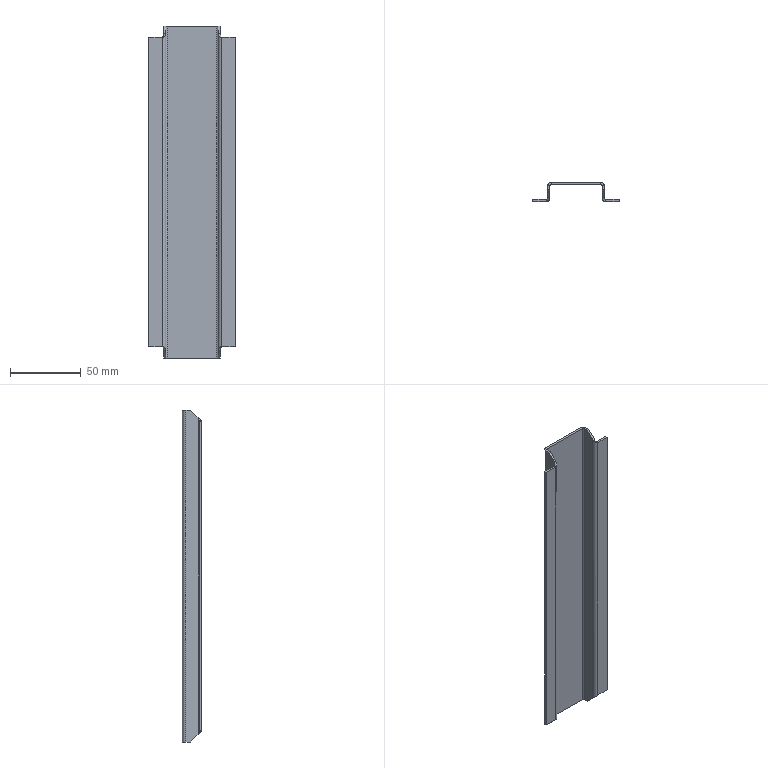Part | SolidWorks | features FlatPattern 1, ICE 1, SMBaseFlange 1, SheetMetal 1 | 1 solid | 42 faces | box 61 x 13.5 x 234.5 mm | volume 28178 mm3 | plane 30 | cylinder 8 | spline 4 | commonest cylinder face diameters 2 x4 5 x4
STEP:
#1=CARTESIAN_POINT('',(22.477,31.708,8.));
#2=VERTEX_POINT('',#1);
#3=CARTESIAN_POINT('',(12.977,31.708,8.));
#4=VERTEX_POINT('',#3);
#5=CARTESIAN_POINT('',(168.477,31.708,8.));
#6=DIRECTION('',(-1.,0.,0.));
#7=VECTOR('',#6,1000.);
#8=LINE('',#5,#7);
#9=EDGE_CURVE('',#2,#4,#8,.T.);
#10=ORIENTED_EDGE('',*,*,#9,.F.);
#11=CARTESIAN_POINT('',(22.477,31.708,226.5));
#12=VERTEX_POINT('',#11);
#13=CARTESIAN_POINT('',(22.477,31.708,234.5));
#14=DIRECTION('',(0.,0.,-1.));
#15=VECTOR('',#14,1000.);
#16=LINE('',#13,#15);
#17=EDGE_CURVE('',#12,#2,#16,.T.);
#18=ORIENTED_EDGE('',*,*,#17,.F.);
#19=CARTESIAN_POINT('',(12.977,31.708,226.5));
#20=VERTEX_POINT('',#19);
#21=CARTESIAN_POINT('',(168.477,31.708,226.5));
#22=DIRECTION('',(-1.,0.,0.));
#23=VECTOR('',#22,1000.);
#24=LINE('',#21,#23);
#25=EDGE_CURVE('',#12,#20,#24,.T.);
#26=ORIENTED_EDGE('',*,*,#25,.T.);
#27=CARTESIAN_POINT('',(12.977,31.708,234.5));
#28=DIRECTION('',(0.,0.,-1.));
#29=VECTOR('',#28,1000.);
#30=LINE('',#27,#29);
#31=EDGE_CURVE('',#20,#4,#30,.T.);
#32=ORIENTED_EDGE('',*,*,#31,.T.);
#33=EDGE_LOOP('',(#10,#18,#26,#32));
#34=FACE_OUTER_BOUND('',#33,.T.);
#35=CARTESIAN_POINT('',(11.977,31.708,234.5));
#36=DIRECTION('',(0.,1.,0.));
#37=DIRECTION('',(0.,0.,1.));
#38=AXIS2_PLACEMENT_3D('',#35,#36,#37);
#39=PLANE('',#38);
#40=ADVANCED_FACE('',(#34),#39,.F.);
#41=ORIENTED_EDGE('',*,*,#17,.T.);
#42=CARTESIAN_POINT('',(22.477,33.208,8.));
#43=VERTEX_POINT('',#42);
#44=CARTESIAN_POINT('',(22.477,31.708,8.));
#45=DIRECTION('',(0.,1.,0.));
#46=VECTOR('',#45,1000.);
#47=LINE('',#44,#46);
#48=EDGE_CURVE('',#2,#43,#47,.T.);
#49=ORIENTED_EDGE('',*,*,#48,.T.);
#50=CARTESIAN_POINT('',(22.477,33.208,226.5));
#51=VERTEX_POINT('',#50);
#52=CARTESIAN_POINT('',(22.477,33.208,234.5));
#53=DIRECTION('',(0.,0.,-1.));
#54=VECTOR('',#53,1000.);
#55=LINE('',#52,#54);
#56=EDGE_CURVE('',#51,#43,#55,.T.);
#57=ORIENTED_EDGE('',*,*,#56,.F.);
#58=CARTESIAN_POINT('',(22.477,31.708,226.5));
#59=DIRECTION('',(0.,1.,0.));
#60=VECTOR('',#59,1000.);
#61=LINE('',#58,#60);
#62=EDGE_CURVE('',#12,#51,#61,.T.);
#63=ORIENTED_EDGE('',*,*,#62,.F.);
#64=EDGE_LOOP('',(#41,#49,#57,#63));
#65=FACE_OUTER_BOUND('',#64,.T.);
#66=CARTESIAN_POINT('',(22.477,33.208,234.5));
#67=DIRECTION('',(1.,0.,0.));
#68=DIRECTION('',(0.,0.,-1.));
#69=AXIS2_PLACEMENT_3D('',#66,#67,#68);
#70=PLANE('',#69);
#71=ADVANCED_FACE('',(#65),#70,.T.);
#72=ORIENTED_EDGE('',*,*,#56,.T.);
#73=CARTESIAN_POINT('',(12.977,33.208,8.));
#74=VERTEX_POINT('',#73);
#75=CARTESIAN_POINT('',(11.977,33.208,8.));
#76=DIRECTION('',(-1.,0.,0.));
#77=VECTOR('',#76,1000.);
#78=LINE('',#75,#77);
#79=EDGE_CURVE('',#43,#74,#78,.T.);
#80=ORIENTED_EDGE('',*,*,#79,.T.);
#81=CARTESIAN_POINT('',(12.977,33.208,226.5));
#82=VERTEX_POINT('',#81);
#83=CARTESIAN_POINT('',(12.977,33.208,234.5));
#84=DIRECTION('',(0.,0.,-1.));
#85=VECTOR('',#84,1000.);
#86=LINE('',#83,#85);
#87=EDGE_CURVE('',#82,#74,#86,.T.);
#88=ORIENTED_EDGE('',*,*,#87,.F.);
#89=CARTESIAN_POINT('',(11.977,33.208,226.5));
#90=DIRECTION('',(-1.,0.,0.));
#91=VECTOR('',#90,1000.);
#92=LINE('',#89,#91);
#93=EDGE_CURVE('',#51,#82,#92,.T.);
#94=ORIENTED_EDGE('',*,*,#93,.F.);
#95=EDGE_LOOP('',(#72,#80,#88,#94));
#96=FACE_OUTER_BOUND('',#95,.T.);
#97=CARTESIAN_POINT('',(11.977,33.208,234.5));
#98=DIRECTION('',(0.,1.,0.));
#99=DIRECTION('',(0.,0.,1.));
#100=AXIS2_PLACEMENT_3D('',#97,#98,#99);
#101=PLANE('',#100);
#102=ADVANCED_FACE('',(#96),#101,.T.);
#103=ORIENTED_EDGE('',*,*,#87,.T.);
#104=CARTESIAN_POINT('',(11.977,34.208,5.5));
#105=VERTEX_POINT('',#104);
#106=CARTESIAN_POINT('',(11.977,34.208,5.5));
#107=CARTESIAN_POINT('',(11.977,33.623,6.964));
#108=CARTESIAN_POINT('',(12.391,33.208,8.));
#109=CARTESIAN_POINT('',(12.977,33.208,8.));
#110=(BOUNDED_CURVE()B_SPLINE_CURVE(3,(#106,#107,#108,#109),.UNSPECIFIED.,.F.,.F.)B_SPLINE_CURVE_WITH_KNOTS((4,4),(1.571,3.142),.UNSPECIFIED.)CURVE()GEOMETRIC_REPRESENTATION_ITEM()RATIONAL_B_SPLINE_CURVE((1.,0.8047,0.8047,1.))REPRESENTATION_ITEM(''));
#111=EDGE_CURVE('',#105,#74,#110,.T.);
#112=ORIENTED_EDGE('',*,*,#111,.F.);
#113=CARTESIAN_POINT('',(11.977,34.208,229.));
#114=VERTEX_POINT('',#113);
#115=CARTESIAN_POINT('',(11.977,34.208,234.5));
#116=DIRECTION('',(0.,0.,-1.));
#117=VECTOR('',#116,1000.);
#118=LINE('',#115,#117);
#119=EDGE_CURVE('',#114,#105,#118,.T.);
#120=ORIENTED_EDGE('',*,*,#119,.F.);
#121=CARTESIAN_POINT('',(12.977,33.208,226.5));
#122=CARTESIAN_POINT('',(12.391,33.208,226.5));
#123=CARTESIAN_POINT('',(11.977,33.623,227.536));
#124=CARTESIAN_POINT('',(11.977,34.208,229.));
#125=(BOUNDED_CURVE()B_SPLINE_CURVE(3,(#121,#122,#123,#124),.UNSPECIFIED.,.F.,.T.)B_SPLINE_CURVE_WITH_KNOTS((4,4),(0.,1.571),.UNSPECIFIED.)CURVE()GEOMETRIC_REPRESENTATION_ITEM()RATIONAL_B_SPLINE_CURVE((1.,0.8047,0.8047,1.))REPRESENTATION_ITEM(''));
#126=EDGE_CURVE('',#82,#114,#125,.T.);
#127=ORIENTED_EDGE('',*,*,#126,.F.);
#128=EDGE_LOOP('',(#103,#112,#120,#127));
#129=FACE_OUTER_BOUND('',#128,.T.);
#130=CARTESIAN_POINT('',(12.977,34.208,234.5));
#131=DIRECTION('',(0.,0.,-1.));
#132=DIRECTION('',(-1.,0.,0.));
#133=AXIS2_PLACEMENT_3D('',#130,#131,#132);
#134=CYLINDRICAL_SURFACE('',#133,1.);
#135=ADVANCED_FACE('',(#129),#134,.F.);
#136=ORIENTED_EDGE('',*,*,#119,.T.);
#137=CARTESIAN_POINT('',(11.977,39.708,0.));
#138=VERTEX_POINT('',#137);
#139=CARTESIAN_POINT('',(11.977,-74.792,114.5));
#140=DIRECTION('',(0.,-0.7071,0.7071));
#141=VECTOR('',#140,1000.);
#142=LINE('',#139,#141);
#143=EDGE_CURVE('',#138,#105,#142,.T.);
#144=ORIENTED_EDGE('',*,*,#143,.F.);
#145=CARTESIAN_POINT('',(11.977,42.708,0.));
#146=VERTEX_POINT('',#145);
#147=CARTESIAN_POINT('',(11.977,45.208,0.));
#148=DIRECTION('',(0.,-1.,0.));
#149=VECTOR('',#148,1000.);
#150=LINE('',#147,#149);
#151=EDGE_CURVE('',#146,#138,#150,.T.);
#152=ORIENTED_EDGE('',*,*,#151,.F.);
#153=CARTESIAN_POINT('',(11.977,42.708,234.5));
#154=VERTEX_POINT('',#153);
#155=CARTESIAN_POINT('',(11.977,42.708,234.5));
#156=DIRECTION('',(0.,0.,-1.));
#157=VECTOR('',#156,1000.);
#158=LINE('',#155,#157);
#159=EDGE_CURVE('',#154,#146,#158,.T.);
#160=ORIENTED_EDGE('',*,*,#159,.F.);
#161=CARTESIAN_POINT('',(11.977,39.708,234.5));
#162=VERTEX_POINT('',#161);
#163=CARTESIAN_POINT('',(11.977,45.208,234.5));
#164=DIRECTION('',(0.,-1.,0.));
#165=VECTOR('',#164,1000.);
#166=LINE('',#163,#165);
#167=EDGE_CURVE('',#154,#162,#166,.T.);
#168=ORIENTED_EDGE('',*,*,#167,.T.);
#169=CARTESIAN_POINT('',(11.977,42.458,237.25));
#170=DIRECTION('',(0.,0.7071,0.7071));
#171=VECTOR('',#170,1000.);
#172=LINE('',#169,#171);
#173=EDGE_CURVE('',#114,#162,#172,.T.);
#174=ORIENTED_EDGE('',*,*,#173,.F.);
#175=EDGE_LOOP('',(#136,#144,#152,#160,#168,#174));
#176=FACE_OUTER_BOUND('',#175,.T.);
#177=CARTESIAN_POINT('',(11.977,45.208,234.5));
#178=DIRECTION('',(1.,0.,0.));
#179=DIRECTION('',(0.,1.,0.));
#180=AXIS2_PLACEMENT_3D('',#177,#178,#179);
#181=PLANE('',#180);
#182=ADVANCED_FACE('',(#176),#181,.T.);
#183=CARTESIAN_POINT('',(10.477,39.708,0.));
#184=VERTEX_POINT('',#183);
#185=CARTESIAN_POINT('',(10.477,34.208,5.5));
#186=VERTEX_POINT('',#185);
#187=CARTESIAN_POINT('',(10.477,-74.792,114.5));
#188=DIRECTION('',(0.,-0.7071,0.7071));
#189=VECTOR('',#188,1000.);
#190=LINE('',#187,#189);
#191=EDGE_CURVE('',#184,#186,#190,.T.);
#192=ORIENTED_EDGE('',*,*,#191,.T.);
#193=CARTESIAN_POINT('',(10.477,34.208,229.));
#194=VERTEX_POINT('',#193);
#195=CARTESIAN_POINT('',(10.477,34.208,234.5));
#196=DIRECTION('',(0.,0.,-1.));
#197=VECTOR('',#196,1000.);
#198=LINE('',#195,#197);
#199=EDGE_CURVE('',#194,#186,#198,.T.);
#200=ORIENTED_EDGE('',*,*,#199,.F.);
#201=CARTESIAN_POINT('',(10.477,39.708,234.5));
#202=VERTEX_POINT('',#201);
#203=CARTESIAN_POINT('',(10.477,42.458,237.25));
#204=DIRECTION('',(0.,0.7071,0.7071));
#205=VECTOR('',#204,1000.);
#206=LINE('',#203,#205);
#207=EDGE_CURVE('',#194,#202,#206,.T.);
#208=ORIENTED_EDGE('',*,*,#207,.T.);
#209=CARTESIAN_POINT('',(10.477,42.708,234.5));
#210=VERTEX_POINT('',#209);
#211=CARTESIAN_POINT('',(10.477,45.208,234.5));
#212=DIRECTION('',(0.,-1.,0.));
#213=VECTOR('',#212,1000.);
#214=LINE('',#211,#213);
#215=EDGE_CURVE('',#210,#202,#214,.T.);
#216=ORIENTED_EDGE('',*,*,#215,.F.);
#217=CARTESIAN_POINT('',(10.477,42.708,0.));
#218=VERTEX_POINT('',#217);
#219=CARTESIAN_POINT('',(10.477,42.708,234.5));
#220=DIRECTION('',(0.,0.,-1.));
#221=VECTOR('',#220,1000.);
#222=LINE('',#219,#221);
#223=EDGE_CURVE('',#210,#218,#222,.T.);
#224=ORIENTED_EDGE('',*,*,#223,.T.);
#225=CARTESIAN_POINT('',(10.477,45.208,0.));
#226=DIRECTION('',(0.,-1.,0.));
#227=VECTOR('',#226,1000.);
#228=LINE('',#225,#227);
#229=EDGE_CURVE('',#218,#184,#228,.T.);
#230=ORIENTED_EDGE('',*,*,#229,.T.);
#231=EDGE_LOOP('',(#192,#200,#208,#216,#224,#230));
#232=FACE_OUTER_BOUND('',#231,.T.);
#233=CARTESIAN_POINT('',(10.477,45.208,234.5));
#234=DIRECTION('',(1.,0.,0.));
#235=DIRECTION('',(0.,1.,0.));
#236=AXIS2_PLACEMENT_3D('',#233,#234,#235);
#237=PLANE('',#236);
#238=ADVANCED_FACE('',(#232),#237,.F.);
#239=CARTESIAN_POINT('',(10.477,34.208,5.5));
#240=CARTESIAN_POINT('',(10.477,32.744,6.964));
#241=CARTESIAN_POINT('',(11.512,31.708,8.));
#242=CARTESIAN_POINT('',(12.977,31.708,8.));
#243=(BOUNDED_CURVE()B_SPLINE_CURVE(3,(#239,#240,#241,#242),.UNSPECIFIED.,.F.,.F.)B_SPLINE_CURVE_WITH_KNOTS((4,4),(1.571,3.142),.UNSPECIFIED.)CURVE()GEOMETRIC_REPRESENTATION_ITEM()RATIONAL_B_SPLINE_CURVE((1.,0.8047,0.8047,1.))REPRESENTATION_ITEM(''));
#244=EDGE_CURVE('',#186,#4,#243,.T.);
#245=ORIENTED_EDGE('',*,*,#244,.T.);
#246=ORIENTED_EDGE('',*,*,#31,.F.);
#247=CARTESIAN_POINT('',(12.977,31.708,226.5));
#248=CARTESIAN_POINT('',(11.512,31.708,226.5));
#249=CARTESIAN_POINT('',(10.477,32.744,227.536));
#250=CARTESIAN_POINT('',(10.477,34.208,229.));
#251=(BOUNDED_CURVE()B_SPLINE_CURVE(3,(#247,#248,#249,#250),.UNSPECIFIED.,.F.,.F.)B_SPLINE_CURVE_WITH_KNOTS((4,4),(0.,1.571),.UNSPECIFIED.)CURVE()GEOMETRIC_REPRESENTATION_ITEM()RATIONAL_B_SPLINE_CURVE((1.,0.8047,0.8047,1.))REPRESENTATION_ITEM(''));
#252=EDGE_CURVE('',#20,#194,#251,.T.);
#253=ORIENTED_EDGE('',*,*,#252,.T.);
#254=ORIENTED_EDGE('',*,*,#199,.T.);
#255=EDGE_LOOP('',(#245,#246,#253,#254));
#256=FACE_OUTER_BOUND('',#255,.T.);
#257=CARTESIAN_POINT('',(12.977,34.208,234.5));
#258=DIRECTION('',(0.,0.,-1.));
#259=DIRECTION('',(-1.,0.,0.));
#260=AXIS2_PLACEMENT_3D('',#257,#258,#259);
#261=CYLINDRICAL_SURFACE('',#260,2.5);
#262=ADVANCED_FACE('',(#256),#261,.T.);
#263=CARTESIAN_POINT('',(-28.023,39.708,0.));
#264=VERTEX_POINT('',#263);
#265=CARTESIAN_POINT('',(-28.023,42.708,0.));
#266=VERTEX_POINT('',#265);
#267=CARTESIAN_POINT('',(-28.023,33.208,0.));
#268=DIRECTION('',(0.,1.,0.));
#269=VECTOR('',#268,1000.);
#270=LINE('',#267,#269);
#271=EDGE_CURVE('',#264,#266,#270,.T.);
#272=ORIENTED_EDGE('',*,*,#271,.F.);
#273=CARTESIAN_POINT('',(-28.023,34.208,5.5));
#274=VERTEX_POINT('',#273);
#275=CARTESIAN_POINT('',(-28.023,-80.792,120.5));
#276=DIRECTION('',(0.,0.7071,-0.7071));
#277=VECTOR('',#276,1000.);
#278=LINE('',#275,#277);
#279=EDGE_CURVE('',#274,#264,#278,.T.);
#280=ORIENTED_EDGE('',*,*,#279,.F.);
#281=CARTESIAN_POINT('',(-28.023,34.208,229.));
#282=VERTEX_POINT('',#281);
#283=CARTESIAN_POINT('',(-28.023,34.208,234.5));
#284=DIRECTION('',(0.,0.,-1.));
#285=VECTOR('',#284,1000.);
#286=LINE('',#283,#285);
#287=EDGE_CURVE('',#282,#274,#286,.T.);
#288=ORIENTED_EDGE('',*,*,#287,.F.);
#289=CARTESIAN_POINT('',(-28.023,39.708,234.5));
#290=VERTEX_POINT('',#289);
#291=CARTESIAN_POINT('',(-28.023,36.458,231.25));
#292=DIRECTION('',(0.,-0.7071,-0.7071));
#293=VECTOR('',#292,1000.);
#294=LINE('',#291,#293);
#295=EDGE_CURVE('',#290,#282,#294,.T.);
#296=ORIENTED_EDGE('',*,*,#295,.F.);
#297=CARTESIAN_POINT('',(-28.023,42.708,234.5));
#298=VERTEX_POINT('',#297);
#299=CARTESIAN_POINT('',(-28.023,33.208,234.5));
#300=DIRECTION('',(0.,1.,0.));
#301=VECTOR('',#300,1000.);
#302=LINE('',#299,#301);
#303=EDGE_CURVE('',#290,#298,#302,.T.);
#304=ORIENTED_EDGE('',*,*,#303,.T.);
#305=CARTESIAN_POINT('',(-28.023,42.708,234.5));
#306=DIRECTION('',(0.,0.,-1.));
#307=VECTOR('',#306,1000.);
#308=LINE('',#305,#307);
#309=EDGE_CURVE('',#298,#266,#308,.T.);
#310=ORIENTED_EDGE('',*,*,#309,.T.);
#311=EDGE_LOOP('',(#272,#280,#288,#296,#304,#310));
#312=FACE_OUTER_BOUND('',#311,.T.);
#313=CARTESIAN_POINT('',(-28.023,33.208,234.5));
#314=DIRECTION('',(-1.,0.,0.));
#315=DIRECTION('',(0.,0.,1.));
#316=AXIS2_PLACEMENT_3D('',#313,#314,#315);
#317=PLANE('',#316);
#318=ADVANCED_FACE('',(#312),#317,.T.);
#319=ORIENTED_EDGE('',*,*,#287,.T.);
#320=CARTESIAN_POINT('',(-29.023,33.208,8.));
#321=VERTEX_POINT('',#320);
#322=CARTESIAN_POINT('',(-29.023,33.208,8.));
#323=CARTESIAN_POINT('',(-28.437,33.208,8.));
#324=CARTESIAN_POINT('',(-28.023,33.623,6.964));
#325=CARTESIAN_POINT('',(-28.023,34.208,5.5));
#326=(BOUNDED_CURVE()B_SPLINE_CURVE(3,(#322,#323,#324,#325),.UNSPECIFIED.,.F.,.F.)B_SPLINE_CURVE_WITH_KNOTS((4,4),(3.142,4.712),.UNSPECIFIED.)CURVE()GEOMETRIC_REPRESENTATION_ITEM()RATIONAL_B_SPLINE_CURVE((1.,0.8047,0.8047,1.))REPRESENTATION_ITEM(''));
#327=EDGE_CURVE('',#321,#274,#326,.T.);
#328=ORIENTED_EDGE('',*,*,#327,.F.);
#329=CARTESIAN_POINT('',(-29.023,33.208,226.5));
#330=VERTEX_POINT('',#329);
#331=CARTESIAN_POINT('',(-29.023,33.208,234.5));
#332=DIRECTION('',(0.,0.,-1.));
#333=VECTOR('',#332,1000.);
#334=LINE('',#331,#333);
#335=EDGE_CURVE('',#330,#321,#334,.T.);
#336=ORIENTED_EDGE('',*,*,#335,.F.);
#337=CARTESIAN_POINT('',(-28.023,34.208,229.));
#338=CARTESIAN_POINT('',(-28.023,33.623,227.536));
#339=CARTESIAN_POINT('',(-28.437,33.208,226.5));
#340=CARTESIAN_POINT('',(-29.023,33.208,226.5));
#341=(BOUNDED_CURVE()B_SPLINE_CURVE(3,(#337,#338,#339,#340),.UNSPECIFIED.,.F.,.T.)B_SPLINE_CURVE_WITH_KNOTS((4,4),(4.712,6.283),.UNSPECIFIED.)CURVE()GEOMETRIC_REPRESENTATION_ITEM()RATIONAL_B_SPLINE_CURVE((1.,0.8047,0.8047,1.))REPRESENTATION_ITEM(''));
#342=EDGE_CURVE('',#282,#330,#341,.T.);
#343=ORIENTED_EDGE('',*,*,#342,.F.);
#344=EDGE_LOOP('',(#319,#328,#336,#343));
#345=FACE_OUTER_BOUND('',#344,.T.);
#346=CARTESIAN_POINT('',(-29.023,34.208,234.5));
#347=DIRECTION('',(0.,0.,-1.));
#348=DIRECTION('',(-1.,0.,0.));
#349=AXIS2_PLACEMENT_3D('',#346,#347,#348);
#350=CYLINDRICAL_SURFACE('',#349,1.);
#351=ADVANCED_FACE('',(#345),#350,.F.);
#352=ORIENTED_EDGE('',*,*,#335,.T.);
#353=CARTESIAN_POINT('',(-38.523,33.208,8.));
#354=VERTEX_POINT('',#353);
#355=CARTESIAN_POINT('',(-38.523,33.208,8.));
#356=DIRECTION('',(-1.,0.,0.));
#357=VECTOR('',#356,1000.);
#358=LINE('',#355,#357);
#359=EDGE_CURVE('',#321,#354,#358,.T.);
#360=ORIENTED_EDGE('',*,*,#359,.T.);
#361=CARTESIAN_POINT('',(-38.523,33.208,226.5));
#362=VERTEX_POINT('',#361);
#363=CARTESIAN_POINT('',(-38.523,33.208,234.5));
#364=DIRECTION('',(0.,0.,-1.));
#365=VECTOR('',#364,1000.);
#366=LINE('',#363,#365);
#367=EDGE_CURVE('',#362,#354,#366,.T.);
#368=ORIENTED_EDGE('',*,*,#367,.F.);
#369=CARTESIAN_POINT('',(-38.523,33.208,226.5));
#370=DIRECTION('',(-1.,0.,0.));
#371=VECTOR('',#370,1000.);
#372=LINE('',#369,#371);
#373=EDGE_CURVE('',#330,#362,#372,.T.);
#374=ORIENTED_EDGE('',*,*,#373,.F.);
#375=EDGE_LOOP('',(#352,#360,#368,#374));
#376=FACE_OUTER_BOUND('',#375,.T.);
#377=CARTESIAN_POINT('',(-38.523,33.208,234.5));
#378=DIRECTION('',(0.,1.,0.));
#379=DIRECTION('',(0.,0.,1.));
#380=AXIS2_PLACEMENT_3D('',#377,#378,#379);
#381=PLANE('',#380);
#382=ADVANCED_FACE('',(#376),#381,.T.);
#383=ORIENTED_EDGE('',*,*,#367,.T.);
#384=CARTESIAN_POINT('',(-38.523,31.708,8.));
#385=VERTEX_POINT('',#384);
#386=CARTESIAN_POINT('',(-38.523,31.708,8.));
#387=DIRECTION('',(0.,1.,0.));
#388=VECTOR('',#387,1000.);
#389=LINE('',#386,#388);
#390=EDGE_CURVE('',#385,#354,#389,.T.);
#391=ORIENTED_EDGE('',*,*,#390,.F.);
#392=CARTESIAN_POINT('',(-38.523,31.708,226.5));
#393=VERTEX_POINT('',#392);
#394=CARTESIAN_POINT('',(-38.523,31.708,234.5));
#395=DIRECTION('',(0.,0.,-1.));
#396=VECTOR('',#395,1000.);
#397=LINE('',#394,#396);
#398=EDGE_CURVE('',#393,#385,#397,.T.);
#399=ORIENTED_EDGE('',*,*,#398,.F.);
#400=CARTESIAN_POINT('',(-38.523,31.708,226.5));
#401=DIRECTION('',(0.,1.,0.));
#402=VECTOR('',#401,1000.);
#403=LINE('',#400,#402);
#404=EDGE_CURVE('',#393,#362,#403,.T.);
#405=ORIENTED_EDGE('',*,*,#404,.T.);
#406=EDGE_LOOP('',(#383,#391,#399,#405));
#407=FACE_OUTER_BOUND('',#406,.T.);
#408=CARTESIAN_POINT('',(-38.523,31.708,234.5));
#409=DIRECTION('',(-1.,0.,0.));
#410=DIRECTION('',(0.,0.,1.));
#411=AXIS2_PLACEMENT_3D('',#408,#409,#410);
#412=PLANE('',#411);
#413=ADVANCED_FACE('',(#407),#412,.T.);
#414=CARTESIAN_POINT('',(-29.023,31.708,8.));
#415=VERTEX_POINT('',#414);
#416=CARTESIAN_POINT('',(168.477,31.708,8.));
#417=DIRECTION('',(-1.,0.,0.));
#418=VECTOR('',#417,1000.);
#419=LINE('',#416,#418);
#420=EDGE_CURVE('',#415,#385,#419,.T.);
#421=ORIENTED_EDGE('',*,*,#420,.F.);
#422=CARTESIAN_POINT('',(-29.023,31.708,226.5));
#423=VERTEX_POINT('',#422);
#424=CARTESIAN_POINT('',(-29.023,31.708,234.5));
#425=DIRECTION('',(0.,0.,-1.));
#426=VECTOR('',#425,1000.);
#427=LINE('',#424,#426);
#428=EDGE_CURVE('',#423,#415,#427,.T.);
#429=ORIENTED_EDGE('',*,*,#428,.F.);
#430=CARTESIAN_POINT('',(168.477,31.708,226.5));
#431=DIRECTION('',(-1.,0.,0.));
#432=VECTOR('',#431,1000.);
#433=LINE('',#430,#432);
#434=EDGE_CURVE('',#423,#393,#433,.T.);
#435=ORIENTED_EDGE('',*,*,#434,.T.);
#436=ORIENTED_EDGE('',*,*,#398,.T.);
#437=EDGE_LOOP('',(#421,#429,#435,#436));
#438=FACE_OUTER_BOUND('',#437,.T.);
#439=CARTESIAN_POINT('',(-38.523,31.708,234.5));
#440=DIRECTION('',(0.,1.,0.));
#441=DIRECTION('',(0.,0.,1.));
#442=AXIS2_PLACEMENT_3D('',#439,#440,#441);
#443=PLANE('',#442);
#444=ADVANCED_FACE('',(#438),#443,.F.);
#445=CARTESIAN_POINT('',(-26.523,34.208,5.5));
#446=VERTEX_POINT('',#445);
#447=CARTESIAN_POINT('',(-29.023,31.708,8.));
#448=CARTESIAN_POINT('',(-27.559,31.708,8.));
#449=CARTESIAN_POINT('',(-26.523,32.744,6.964));
#450=CARTESIAN_POINT('',(-26.523,34.208,5.5));
#451=(BOUNDED_CURVE()B_SPLINE_CURVE(3,(#447,#448,#449,#450),.UNSPECIFIED.,.F.,.F.)B_SPLINE_CURVE_WITH_KNOTS((4,4),(3.142,4.712),.UNSPECIFIED.)CURVE()GEOMETRIC_REPRESENTATION_ITEM()RATIONAL_B_SPLINE_CURVE((1.,0.8047,0.8047,1.))REPRESENTATION_ITEM(''));
#452=EDGE_CURVE('',#415,#446,#451,.T.);
#453=ORIENTED_EDGE('',*,*,#452,.T.);
#454=CARTESIAN_POINT('',(-26.523,34.208,229.));
#455=VERTEX_POINT('',#454);
#456=CARTESIAN_POINT('',(-26.523,34.208,234.5));
#457=DIRECTION('',(0.,0.,-1.));
#458=VECTOR('',#457,1000.);
#459=LINE('',#456,#458);
#460=EDGE_CURVE('',#455,#446,#459,.T.);
#461=ORIENTED_EDGE('',*,*,#460,.F.);
#462=CARTESIAN_POINT('',(-26.523,34.208,229.));
#463=CARTESIAN_POINT('',(-26.523,32.744,227.536));
#464=CARTESIAN_POINT('',(-27.559,31.708,226.5));
#465=CARTESIAN_POINT('',(-29.023,31.708,226.5));
#466=(BOUNDED_CURVE()B_SPLINE_CURVE(3,(#462,#463,#464,#465),.UNSPECIFIED.,.F.,.T.)B_SPLINE_CURVE_WITH_KNOTS((4,4),(4.712,6.283),.UNSPECIFIED.)CURVE()GEOMETRIC_REPRESENTATION_ITEM()RATIONAL_B_SPLINE_CURVE((1.,0.8047,0.8047,1.))REPRESENTATION_ITEM(''));
#467=EDGE_CURVE('',#455,#423,#466,.T.);
#468=ORIENTED_EDGE('',*,*,#467,.T.);
#469=ORIENTED_EDGE('',*,*,#428,.T.);
#470=EDGE_LOOP('',(#453,#461,#468,#469));
#471=FACE_OUTER_BOUND('',#470,.T.);
#472=CARTESIAN_POINT('',(-29.023,34.208,234.5));
#473=DIRECTION('',(0.,0.,-1.));
#474=DIRECTION('',(-1.,0.,0.));
#475=AXIS2_PLACEMENT_3D('',#472,#473,#474);
#476=CYLINDRICAL_SURFACE('',#475,2.5);
#477=ADVANCED_FACE('',(#471),#476,.T.);
#478=CARTESIAN_POINT('',(-26.523,39.708,0.));
#479=VERTEX_POINT('',#478);
#480=CARTESIAN_POINT('',(-26.523,-80.792,120.5));
#481=DIRECTION('',(0.,0.7071,-0.7071));
#482=VECTOR('',#481,1000.);
#483=LINE('',#480,#482);
#484=EDGE_CURVE('',#446,#479,#483,.T.);
#485=ORIENTED_EDGE('',*,*,#484,.T.);
#486=CARTESIAN_POINT('',(-26.523,42.708,0.));
#487=VERTEX_POINT('',#486);
#488=CARTESIAN_POINT('',(-26.523,33.208,0.));
#489=DIRECTION('',(0.,1.,0.));
#490=VECTOR('',#489,1000.);
#491=LINE('',#488,#490);
#492=EDGE_CURVE('',#479,#487,#491,.T.);
#493=ORIENTED_EDGE('',*,*,#492,.T.);
#494=CARTESIAN_POINT('',(-26.523,42.708,234.5));
#495=VERTEX_POINT('',#494);
#496=CARTESIAN_POINT('',(-26.523,42.708,234.5));
#497=DIRECTION('',(0.,0.,-1.));
#498=VECTOR('',#497,1000.);
#499=LINE('',#496,#498);
#500=EDGE_CURVE('',#495,#487,#499,.T.);
#501=ORIENTED_EDGE('',*,*,#500,.F.);
#502=CARTESIAN_POINT('',(-26.523,39.708,234.5));
#503=VERTEX_POINT('',#502);
#504=CARTESIAN_POINT('',(-26.523,33.208,234.5));
#505=DIRECTION('',(0.,1.,0.));
#506=VECTOR('',#505,1000.);
#507=LINE('',#504,#506);
#508=EDGE_CURVE('',#503,#495,#507,.T.);
#509=ORIENTED_EDGE('',*,*,#508,.F.);
#510=CARTESIAN_POINT('',(-26.523,36.458,231.25));
#511=DIRECTION('',(0.,-0.7071,-0.7071));
#512=VECTOR('',#511,1000.);
#513=LINE('',#510,#512);
#514=EDGE_CURVE('',#503,#455,#513,.T.);
#515=ORIENTED_EDGE('',*,*,#514,.T.);
#516=ORIENTED_EDGE('',*,*,#460,.T.);
#517=EDGE_LOOP('',(#485,#493,#501,#509,#515,#516));
#518=FACE_OUTER_BOUND('',#517,.T.);
#519=CARTESIAN_POINT('',(-26.523,33.208,234.5));
#520=DIRECTION('',(-1.,0.,0.));
#521=DIRECTION('',(0.,0.,1.));
#522=AXIS2_PLACEMENT_3D('',#519,#520,#521);
#523=PLANE('',#522);
#524=ADVANCED_FACE('',(#518),#523,.F.);
#525=ORIENTED_EDGE('',*,*,#303,.F.);
#526=CARTESIAN_POINT('',(-28.023,39.708,234.5));
#527=DIRECTION('',(1.,0.,0.));
#528=VECTOR('',#527,1000.);
#529=LINE('',#526,#528);
#530=EDGE_CURVE('',#290,#503,#529,.T.);
#531=ORIENTED_EDGE('',*,*,#530,.T.);
#532=ORIENTED_EDGE('',*,*,#508,.T.);
#533=CARTESIAN_POINT('',(-26.523,42.708,234.5));
#534=DIRECTION('',(-1.,0.,0.));
#535=VECTOR('',#534,1000.);
#536=LINE('',#533,#535);
#537=EDGE_CURVE('',#495,#298,#536,.T.);
#538=ORIENTED_EDGE('',*,*,#537,.T.);
#539=EDGE_LOOP('',(#525,#531,#532,#538));
#540=FACE_OUTER_BOUND('',#539,.T.);
#541=CARTESIAN_POINT('',(-29.023,31.708,234.5));
#542=DIRECTION('',(0.,0.,1.));
#543=DIRECTION('',(1.,0.,0.));
#544=AXIS2_PLACEMENT_3D('',#541,#542,#543);
#545=PLANE('',#544);
#546=ADVANCED_FACE('',(#540),#545,.T.);
#547=CARTESIAN_POINT('',(-25.523,45.208,234.5));
#548=VERTEX_POINT('',#547);
#549=CARTESIAN_POINT('',(-25.523,43.708,234.5));
#550=VERTEX_POINT('',#549);
#551=CARTESIAN_POINT('',(-25.523,45.208,234.5));
#552=DIRECTION('',(0.,-1.,0.));
#553=VECTOR('',#552,1000.);
#554=LINE('',#551,#553);
#555=EDGE_CURVE('',#548,#550,#554,.T.);
#556=ORIENTED_EDGE('',*,*,#555,.F.);
#557=CARTESIAN_POINT('',(-25.523,42.708,234.5));
#558=DIRECTION('',(0.,0.,-1.));
#559=DIRECTION('',(1.,0.,0.));
#560=AXIS2_PLACEMENT_3D('',#557,#558,#559);
#561=CIRCLE('',#560,2.5);
#562=EDGE_CURVE('',#298,#548,#561,.T.);
#563=ORIENTED_EDGE('',*,*,#562,.F.);
#564=ORIENTED_EDGE('',*,*,#537,.F.);
#565=CARTESIAN_POINT('',(-25.523,42.708,234.5));
#566=DIRECTION('',(0.,0.,-1.));
#567=DIRECTION('',(1.,0.,0.));
#568=AXIS2_PLACEMENT_3D('',#565,#566,#567);
#569=CIRCLE('',#568,1.);
#570=EDGE_CURVE('',#495,#550,#569,.T.);
#571=ORIENTED_EDGE('',*,*,#570,.T.);
#572=EDGE_LOOP('',(#556,#563,#564,#571));
#573=FACE_OUTER_BOUND('',#572,.T.);
#574=CARTESIAN_POINT('',(-25.523,45.208,234.5));
#575=DIRECTION('',(0.,0.,1.));
#576=DIRECTION('',(1.,0.,0.));
#577=AXIS2_PLACEMENT_3D('',#574,#575,#576);
#578=PLANE('',#577);
#579=ADVANCED_FACE('',(#573),#578,.T.);
#580=CARTESIAN_POINT('',(9.477,45.208,234.5));
#581=VERTEX_POINT('',#580);
#582=CARTESIAN_POINT('',(-28.023,45.208,234.5));
#583=DIRECTION('',(1.,0.,0.));
#584=VECTOR('',#583,1000.);
#585=LINE('',#582,#584);
#586=EDGE_CURVE('',#548,#581,#585,.T.);
#587=ORIENTED_EDGE('',*,*,#586,.F.);
#588=ORIENTED_EDGE('',*,*,#555,.T.);
#589=CARTESIAN_POINT('',(9.477,43.708,234.5));
#590=VERTEX_POINT('',#589);
#591=CARTESIAN_POINT('',(-28.023,43.708,234.5));
#592=DIRECTION('',(1.,0.,0.));
#593=VECTOR('',#592,1000.);
#594=LINE('',#591,#593);
#595=EDGE_CURVE('',#550,#590,#594,.T.);
#596=ORIENTED_EDGE('',*,*,#595,.T.);
#597=CARTESIAN_POINT('',(9.477,43.708,234.5));
#598=DIRECTION('',(0.,1.,0.));
#599=VECTOR('',#598,1000.);
#600=LINE('',#597,#599);
#601=EDGE_CURVE('',#590,#581,#600,.T.);
#602=ORIENTED_EDGE('',*,*,#601,.T.);
#603=EDGE_LOOP('',(#587,#588,#596,#602));
#604=FACE_OUTER_BOUND('',#603,.T.);
#605=CARTESIAN_POINT('',(-26.523,42.708,234.5));
#606=DIRECTION('',(0.,0.,1.));
#607=DIRECTION('',(1.,0.,0.));
#608=AXIS2_PLACEMENT_3D('',#605,#606,#607);
#609=PLANE('',#608);
#610=ADVANCED_FACE('',(#604),#609,.T.);
#611=CARTESIAN_POINT('',(-28.023,42.708,0.));
#612=DIRECTION('',(1.,0.,0.));
#613=VECTOR('',#612,1000.);
#614=LINE('',#611,#613);
#615=EDGE_CURVE('',#266,#487,#614,.T.);
#616=ORIENTED_EDGE('',*,*,#615,.F.);
#617=CARTESIAN_POINT('',(-25.523,45.208,0.));
#618=VERTEX_POINT('',#617);
#619=CARTESIAN_POINT('',(-25.523,42.708,0.));
#620=DIRECTION('',(0.,0.,-1.));
#621=DIRECTION('',(1.,0.,0.));
#622=AXIS2_PLACEMENT_3D('',#619,#620,#621);
#623=CIRCLE('',#622,2.5);
#624=EDGE_CURVE('',#266,#618,#623,.T.);
#625=ORIENTED_EDGE('',*,*,#624,.T.);
#626=CARTESIAN_POINT('',(-25.523,43.708,0.));
#627=VERTEX_POINT('',#626);
#628=CARTESIAN_POINT('',(-25.523,43.708,0.));
#629=DIRECTION('',(0.,1.,0.));
#630=VECTOR('',#629,1000.);
#631=LINE('',#628,#630);
#632=EDGE_CURVE('',#627,#618,#631,.T.);
#633=ORIENTED_EDGE('',*,*,#632,.F.);
#634=CARTESIAN_POINT('',(-25.523,42.708,0.));
#635=DIRECTION('',(0.,0.,-1.));
#636=DIRECTION('',(1.,0.,0.));
#637=AXIS2_PLACEMENT_3D('',#634,#635,#636);
#638=CIRCLE('',#637,1.);
#639=EDGE_CURVE('',#487,#627,#638,.T.);
#640=ORIENTED_EDGE('',*,*,#639,.F.);
#641=EDGE_LOOP('',(#616,#625,#633,#640));
#642=FACE_OUTER_BOUND('',#641,.T.);
#643=CARTESIAN_POINT('',(-28.023,42.708,0.));
#644=DIRECTION('',(0.,0.,-1.));
#645=DIRECTION('',(-1.,0.,0.));
#646=AXIS2_PLACEMENT_3D('',#643,#644,#645);
#647=PLANE('',#646);
#648=ADVANCED_FACE('',(#642),#647,.T.);
#649=ORIENTED_EDGE('',*,*,#492,.F.);
#650=CARTESIAN_POINT('',(-28.023,39.708,0.));
#651=DIRECTION('',(1.,0.,0.));
#652=VECTOR('',#651,1000.);
#653=LINE('',#650,#652);
#654=EDGE_CURVE('',#264,#479,#653,.T.);
#655=ORIENTED_EDGE('',*,*,#654,.F.);
#656=ORIENTED_EDGE('',*,*,#271,.T.);
#657=ORIENTED_EDGE('',*,*,#615,.T.);
#658=EDGE_LOOP('',(#649,#655,#656,#657));
#659=FACE_OUTER_BOUND('',#658,.T.);
#660=CARTESIAN_POINT('',(-25.523,43.708,0.));
#661=DIRECTION('',(0.,0.,-1.));
#662=DIRECTION('',(-1.,0.,0.));
#663=AXIS2_PLACEMENT_3D('',#660,#661,#662);
#664=PLANE('',#663);
#665=ADVANCED_FACE('',(#659),#664,.T.);
#666=CARTESIAN_POINT('',(11.977,42.708,234.5));
#667=DIRECTION('',(-1.,0.,0.));
#668=VECTOR('',#667,1000.);
#669=LINE('',#666,#668);
#670=EDGE_CURVE('',#154,#210,#669,.T.);
#671=ORIENTED_EDGE('',*,*,#670,.F.);
#672=CARTESIAN_POINT('',(9.477,42.708,234.5));
#673=DIRECTION('',(0.,0.,-1.));
#674=DIRECTION('',(1.,0.,0.));
#675=AXIS2_PLACEMENT_3D('',#672,#673,#674);
#676=CIRCLE('',#675,2.5);
#677=EDGE_CURVE('',#581,#154,#676,.T.);
#678=ORIENTED_EDGE('',*,*,#677,.F.);
#679=ORIENTED_EDGE('',*,*,#601,.F.);
#680=CARTESIAN_POINT('',(9.477,42.708,234.5));
#681=DIRECTION('',(0.,0.,-1.));
#682=DIRECTION('',(1.,0.,0.));
#683=AXIS2_PLACEMENT_3D('',#680,#681,#682);
#684=CIRCLE('',#683,1.);
#685=EDGE_CURVE('',#590,#210,#684,.T.);
#686=ORIENTED_EDGE('',*,*,#685,.T.);
#687=EDGE_LOOP('',(#671,#678,#679,#686));
#688=FACE_OUTER_BOUND('',#687,.T.);
#689=CARTESIAN_POINT('',(11.977,42.708,234.5));
#690=DIRECTION('',(0.,0.,1.));
#691=DIRECTION('',(1.,0.,0.));
#692=AXIS2_PLACEMENT_3D('',#689,#690,#691);
#693=PLANE('',#692);
#694=ADVANCED_FACE('',(#688),#693,.T.);
#695=ORIENTED_EDGE('',*,*,#215,.T.);
#696=CARTESIAN_POINT('',(10.477,39.708,234.5));
#697=DIRECTION('',(1.,0.,0.));
#698=VECTOR('',#697,1000.);
#699=LINE('',#696,#698);
#700=EDGE_CURVE('',#202,#162,#699,.T.);
#701=ORIENTED_EDGE('',*,*,#700,.T.);
#702=ORIENTED_EDGE('',*,*,#167,.F.);
#703=ORIENTED_EDGE('',*,*,#670,.T.);
#704=EDGE_LOOP('',(#695,#701,#702,#703));
#705=FACE_OUTER_BOUND('',#704,.T.);
#706=CARTESIAN_POINT('',(9.477,43.708,234.5));
#707=DIRECTION('',(0.,0.,1.));
#708=DIRECTION('',(1.,0.,0.));
#709=AXIS2_PLACEMENT_3D('',#706,#707,#708);
#710=PLANE('',#709);
#711=ADVANCED_FACE('',(#705),#710,.T.);
#712=CARTESIAN_POINT('',(9.477,45.208,0.));
#713=VERTEX_POINT('',#712);
#714=CARTESIAN_POINT('',(9.477,43.708,0.));
#715=VERTEX_POINT('',#714);
#716=CARTESIAN_POINT('',(9.477,45.208,0.));
#717=DIRECTION('',(0.,-1.,0.));
#718=VECTOR('',#717,1000.);
#719=LINE('',#716,#718);
#720=EDGE_CURVE('',#713,#715,#719,.T.);
#721=ORIENTED_EDGE('',*,*,#720,.F.);
#722=CARTESIAN_POINT('',(9.477,42.708,0.));
#723=DIRECTION('',(0.,0.,-1.));
#724=DIRECTION('',(1.,0.,0.));
#725=AXIS2_PLACEMENT_3D('',#722,#723,#724);
#726=CIRCLE('',#725,2.5);
#727=EDGE_CURVE('',#713,#146,#726,.T.);
#728=ORIENTED_EDGE('',*,*,#727,.T.);
#729=CARTESIAN_POINT('',(10.477,42.708,0.));
#730=DIRECTION('',(1.,0.,0.));
#731=VECTOR('',#730,1000.);
#732=LINE('',#729,#731);
#733=EDGE_CURVE('',#218,#146,#732,.T.);
#734=ORIENTED_EDGE('',*,*,#733,.F.);
#735=CARTESIAN_POINT('',(9.477,42.708,0.));
#736=DIRECTION('',(0.,0.,-1.));
#737=DIRECTION('',(1.,0.,0.));
#738=AXIS2_PLACEMENT_3D('',#735,#736,#737);
#739=CIRCLE('',#738,1.);
#740=EDGE_CURVE('',#715,#218,#739,.T.);
#741=ORIENTED_EDGE('',*,*,#740,.F.);
#742=EDGE_LOOP('',(#721,#728,#734,#741));
#743=FACE_OUTER_BOUND('',#742,.T.);
#744=CARTESIAN_POINT('',(9.477,45.208,0.));
#745=DIRECTION('',(0.,0.,-1.));
#746=DIRECTION('',(-1.,0.,0.));
#747=AXIS2_PLACEMENT_3D('',#744,#745,#746);
#748=PLANE('',#747);
#749=ADVANCED_FACE('',(#743),#748,.T.);
#750=CARTESIAN_POINT('',(-28.023,45.208,0.));
#751=DIRECTION('',(1.,0.,0.));
#752=VECTOR('',#751,1000.);
#753=LINE('',#750,#752);
#754=EDGE_CURVE('',#618,#713,#753,.T.);
#755=ORIENTED_EDGE('',*,*,#754,.T.);
#756=ORIENTED_EDGE('',*,*,#720,.T.);
#757=CARTESIAN_POINT('',(-28.023,43.708,0.));
#758=DIRECTION('',(1.,0.,0.));
#759=VECTOR('',#758,1000.);
#760=LINE('',#757,#759);
#761=EDGE_CURVE('',#627,#715,#760,.T.);
#762=ORIENTED_EDGE('',*,*,#761,.F.);
#763=ORIENTED_EDGE('',*,*,#632,.T.);
#764=EDGE_LOOP('',(#755,#756,#762,#763));
#765=FACE_OUTER_BOUND('',#764,.T.);
#766=CARTESIAN_POINT('',(10.477,42.708,0.));
#767=DIRECTION('',(0.,0.,-1.));
#768=DIRECTION('',(-1.,0.,0.));
#769=AXIS2_PLACEMENT_3D('',#766,#767,#768);
#770=PLANE('',#769);
#771=ADVANCED_FACE('',(#765),#770,.T.);
#772=ORIENTED_EDGE('',*,*,#151,.T.);
#773=CARTESIAN_POINT('',(11.977,39.708,0.));
#774=DIRECTION('',(-1.,0.,0.));
#775=VECTOR('',#774,1000.);
#776=LINE('',#773,#775);
#777=EDGE_CURVE('',#138,#184,#776,.T.);
#778=ORIENTED_EDGE('',*,*,#777,.T.);
#779=ORIENTED_EDGE('',*,*,#229,.F.);
#780=ORIENTED_EDGE('',*,*,#733,.T.);
#781=EDGE_LOOP('',(#772,#778,#779,#780));
#782=FACE_OUTER_BOUND('',#781,.T.);
#783=CARTESIAN_POINT('',(12.977,31.708,0.));
#784=DIRECTION('',(0.,0.,-1.));
#785=DIRECTION('',(-1.,0.,0.));
#786=AXIS2_PLACEMENT_3D('',#783,#784,#785);
#787=PLANE('',#786);
#788=ADVANCED_FACE('',(#782),#787,.T.);
#789=ORIENTED_EDGE('',*,*,#727,.F.);
#790=CARTESIAN_POINT('',(9.477,45.208,234.5));
#791=DIRECTION('',(0.,0.,-1.));
#792=VECTOR('',#791,1000.);
#793=LINE('',#790,#792);
#794=EDGE_CURVE('',#581,#713,#793,.T.);
#795=ORIENTED_EDGE('',*,*,#794,.F.);
#796=ORIENTED_EDGE('',*,*,#677,.T.);
#797=ORIENTED_EDGE('',*,*,#159,.T.);
#798=EDGE_LOOP('',(#789,#795,#796,#797));
#799=FACE_OUTER_BOUND('',#798,.T.);
#800=CARTESIAN_POINT('',(9.477,42.708,234.5));
#801=DIRECTION('',(0.,0.,-1.));
#802=DIRECTION('',(-1.,0.,0.));
#803=AXIS2_PLACEMENT_3D('',#800,#801,#802);
#804=CYLINDRICAL_SURFACE('',#803,2.5);
#805=ADVANCED_FACE('',(#799),#804,.T.);
#806=ORIENTED_EDGE('',*,*,#754,.F.);
#807=CARTESIAN_POINT('',(-25.523,45.208,234.5));
#808=DIRECTION('',(0.,0.,-1.));
#809=VECTOR('',#808,1000.);
#810=LINE('',#807,#809);
#811=EDGE_CURVE('',#548,#618,#810,.T.);
#812=ORIENTED_EDGE('',*,*,#811,.F.);
#813=ORIENTED_EDGE('',*,*,#586,.T.);
#814=ORIENTED_EDGE('',*,*,#794,.T.);
#815=EDGE_LOOP('',(#806,#812,#813,#814));
#816=FACE_OUTER_BOUND('',#815,.T.);
#817=CARTESIAN_POINT('',(-28.023,45.208,234.5));
#818=DIRECTION('',(0.,1.,0.));
#819=DIRECTION('',(0.,0.,1.));
#820=AXIS2_PLACEMENT_3D('',#817,#818,#819);
#821=PLANE('',#820);
#822=ADVANCED_FACE('',(#816),#821,.T.);
#823=ORIENTED_EDGE('',*,*,#624,.F.);
#824=ORIENTED_EDGE('',*,*,#309,.F.);
#825=ORIENTED_EDGE('',*,*,#562,.T.);
#826=ORIENTED_EDGE('',*,*,#811,.T.);
#827=EDGE_LOOP('',(#823,#824,#825,#826));
#828=FACE_OUTER_BOUND('',#827,.T.);
#829=CARTESIAN_POINT('',(-25.523,42.708,234.5));
#830=DIRECTION('',(0.,0.,-1.));
#831=DIRECTION('',(-1.,0.,0.));
#832=AXIS2_PLACEMENT_3D('',#829,#830,#831);
#833=CYLINDRICAL_SURFACE('',#832,2.5);
#834=ADVANCED_FACE('',(#828),#833,.T.);
#835=ORIENTED_EDGE('',*,*,#639,.T.);
#836=CARTESIAN_POINT('',(-25.523,43.708,234.5));
#837=DIRECTION('',(0.,0.,-1.));
#838=VECTOR('',#837,1000.);
#839=LINE('',#836,#838);
#840=EDGE_CURVE('',#550,#627,#839,.T.);
#841=ORIENTED_EDGE('',*,*,#840,.F.);
#842=ORIENTED_EDGE('',*,*,#570,.F.);
#843=ORIENTED_EDGE('',*,*,#500,.T.);
#844=EDGE_LOOP('',(#835,#841,#842,#843));
#845=FACE_OUTER_BOUND('',#844,.T.);
#846=CARTESIAN_POINT('',(-25.523,42.708,234.5));
#847=DIRECTION('',(0.,0.,-1.));
#848=DIRECTION('',(-1.,0.,0.));
#849=AXIS2_PLACEMENT_3D('',#846,#847,#848);
#850=CYLINDRICAL_SURFACE('',#849,1.);
#851=ADVANCED_FACE('',(#845),#850,.F.);
#852=ORIENTED_EDGE('',*,*,#761,.T.);
#853=CARTESIAN_POINT('',(9.477,43.708,234.5));
#854=DIRECTION('',(0.,0.,-1.));
#855=VECTOR('',#854,1000.);
#856=LINE('',#853,#855);
#857=EDGE_CURVE('',#590,#715,#856,.T.);
#858=ORIENTED_EDGE('',*,*,#857,.F.);
#859=ORIENTED_EDGE('',*,*,#595,.F.);
#860=ORIENTED_EDGE('',*,*,#840,.T.);
#861=EDGE_LOOP('',(#852,#858,#859,#860));
#862=FACE_OUTER_BOUND('',#861,.T.);
#863=CARTESIAN_POINT('',(-28.023,43.708,234.5));
#864=DIRECTION('',(0.,1.,0.));
#865=DIRECTION('',(0.,0.,1.));
#866=AXIS2_PLACEMENT_3D('',#863,#864,#865);
#867=PLANE('',#866);
#868=ADVANCED_FACE('',(#862),#867,.F.);
#869=ORIENTED_EDGE('',*,*,#740,.T.);
#870=ORIENTED_EDGE('',*,*,#223,.F.);
#871=ORIENTED_EDGE('',*,*,#685,.F.);
#872=ORIENTED_EDGE('',*,*,#857,.T.);
#873=EDGE_LOOP('',(#869,#870,#871,#872));
#874=FACE_OUTER_BOUND('',#873,.T.);
#875=CARTESIAN_POINT('',(9.477,42.708,234.5));
#876=DIRECTION('',(0.,0.,-1.));
#877=DIRECTION('',(-1.,0.,0.));
#878=AXIS2_PLACEMENT_3D('',#875,#876,#877);
#879=CYLINDRICAL_SURFACE('',#878,1.);
#880=ADVANCED_FACE('',(#874),#879,.F.);
#881=ORIENTED_EDGE('',*,*,#295,.T.);
#882=CARTESIAN_POINT('',(-28.023,34.208,229.));
#883=DIRECTION('',(1.,0.,0.));
#884=VECTOR('',#883,1000.);
#885=LINE('',#882,#884);
#886=EDGE_CURVE('',#282,#455,#885,.T.);
#887=ORIENTED_EDGE('',*,*,#886,.T.);
#888=ORIENTED_EDGE('',*,*,#514,.F.);
#889=ORIENTED_EDGE('',*,*,#530,.F.);
#890=EDGE_LOOP('',(#881,#887,#888,#889));
#891=FACE_OUTER_BOUND('',#890,.T.);
#892=CARTESIAN_POINT('',(-28.023,36.458,231.25));
#893=DIRECTION('',(0.,0.7071,-0.7071));
#894=DIRECTION('',(0.,-0.7071,-0.7071));
#895=AXIS2_PLACEMENT_3D('',#892,#893,#894);
#896=PLANE('',#895);
#897=ADVANCED_FACE('',(#891),#896,.F.);
#898=ORIENTED_EDGE('',*,*,#404,.F.);
#899=ORIENTED_EDGE('',*,*,#434,.F.);
#900=CARTESIAN_POINT('',(-29.023,31.708,226.5));
#901=DIRECTION('',(0.,1.,0.));
#902=VECTOR('',#901,1000.);
#903=LINE('',#900,#902);
#904=EDGE_CURVE('',#423,#330,#903,.T.);
#905=ORIENTED_EDGE('',*,*,#904,.T.);
#906=ORIENTED_EDGE('',*,*,#373,.T.);
#907=EDGE_LOOP('',(#898,#899,#905,#906));
#908=FACE_OUTER_BOUND('',#907,.T.);
#909=CARTESIAN_POINT('',(168.477,31.708,226.5));
#910=DIRECTION('',(0.,0.,-1.));
#911=DIRECTION('',(-1.,0.,0.));
#912=AXIS2_PLACEMENT_3D('',#909,#910,#911);
#913=PLANE('',#912);
#914=ADVANCED_FACE('',(#908),#913,.F.);
#915=ORIENTED_EDGE('',*,*,#904,.F.);
#916=ORIENTED_EDGE('',*,*,#467,.F.);
#917=ORIENTED_EDGE('',*,*,#886,.F.);
#918=ORIENTED_EDGE('',*,*,#342,.T.);
#919=EDGE_LOOP('',(#915,#916,#917,#918));
#920=FACE_OUTER_BOUND('',#919,.T.);
#921=CARTESIAN_POINT('',(-29.023,33.208,226.5));
#922=CARTESIAN_POINT('',(-29.023,32.708,226.5));
#923=CARTESIAN_POINT('',(-29.023,32.208,226.5));
#924=CARTESIAN_POINT('',(-29.023,31.708,226.5));
#925=CARTESIAN_POINT('',(-31.023,33.208,226.5));
#926=CARTESIAN_POINT('',(-32.023,32.708,226.5));
#927=CARTESIAN_POINT('',(-33.023,32.208,226.5));
#928=CARTESIAN_POINT('',(-34.023,31.708,226.5));
#929=CARTESIAN_POINT('',(-31.023,35.208,231.5));
#930=CARTESIAN_POINT('',(-32.023,35.708,231.5));
#931=CARTESIAN_POINT('',(-33.023,36.208,231.5));
#932=CARTESIAN_POINT('',(-34.023,36.708,231.5));
#933=CARTESIAN_POINT('',(-29.023,35.208,231.5));
#934=CARTESIAN_POINT('',(-29.023,35.708,231.5));
#935=CARTESIAN_POINT('',(-29.023,36.208,231.5));
#936=CARTESIAN_POINT('',(-29.023,36.708,231.5));
#937=CARTESIAN_POINT('',(-27.023,35.208,231.5));
#938=CARTESIAN_POINT('',(-26.023,35.708,231.5));
#939=CARTESIAN_POINT('',(-25.023,36.208,231.5));
#940=CARTESIAN_POINT('',(-24.023,36.708,231.5));
#941=CARTESIAN_POINT('',(-27.023,33.208,226.5));
#942=CARTESIAN_POINT('',(-26.023,32.708,226.5));
#943=CARTESIAN_POINT('',(-25.023,32.208,226.5));
#944=CARTESIAN_POINT('',(-24.023,31.708,226.5));
#945=CARTESIAN_POINT('',(-29.023,33.208,226.5));
#946=CARTESIAN_POINT('',(-29.023,32.708,226.5));
#947=CARTESIAN_POINT('',(-29.023,32.208,226.5));
#948=CARTESIAN_POINT('',(-29.023,31.708,226.5));
#949=(BOUNDED_SURFACE()B_SPLINE_SURFACE(3,3,((#921,#922,#923,#924),(#925,#926,#927,#928),(#929,#930,#931,#932),(#933,#934,#935,#936),(#937,#938,#939,#940),(#941,#942,#943,#944),(#945,#946,#947,#948)),.UNSPECIFIED.,.T.,.F.,.T.)B_SPLINE_SURFACE_WITH_KNOTS((4,3,4),(4,4),(0.,0.5,1.),(0.,1.),.UNSPECIFIED.)GEOMETRIC_REPRESENTATION_ITEM()RATIONAL_B_SPLINE_SURFACE(((1.,1.,1.,1.),(0.3333,0.3333,0.3333,0.3333),(0.3333,0.3333,0.3333,0.3333),(1.,1.,1.,1.),(0.3333,0.3333,0.3333,0.3333),(0.3333,0.3333,0.3333,0.3333),(1.,1.,1.,1.)))REPRESENTATION_ITEM('')SURFACE());
#950=ADVANCED_FACE('',(#920),#949,.T.);
#951=ORIENTED_EDGE('',*,*,#279,.T.);
#952=ORIENTED_EDGE('',*,*,#654,.T.);
#953=ORIENTED_EDGE('',*,*,#484,.F.);
#954=CARTESIAN_POINT('',(-28.023,34.208,5.5));
#955=DIRECTION('',(1.,0.,0.));
#956=VECTOR('',#955,1000.);
#957=LINE('',#954,#956);
#958=EDGE_CURVE('',#274,#446,#957,.T.);
#959=ORIENTED_EDGE('',*,*,#958,.F.);
#960=EDGE_LOOP('',(#951,#952,#953,#959));
#961=FACE_OUTER_BOUND('',#960,.T.);
#962=CARTESIAN_POINT('',(-28.023,-80.792,120.5));
#963=DIRECTION('',(0.,0.7071,0.7071));
#964=DIRECTION('',(0.,0.7071,-0.7071));
#965=AXIS2_PLACEMENT_3D('',#962,#963,#964);
#966=PLANE('',#965);
#967=ADVANCED_FACE('',(#961),#966,.F.);
#968=CARTESIAN_POINT('',(-29.023,31.708,8.));
#969=DIRECTION('',(0.,1.,0.));
#970=VECTOR('',#969,1000.);
#971=LINE('',#968,#970);
#972=EDGE_CURVE('',#415,#321,#971,.T.);
#973=ORIENTED_EDGE('',*,*,#972,.F.);
#974=ORIENTED_EDGE('',*,*,#420,.T.);
#975=ORIENTED_EDGE('',*,*,#390,.T.);
#976=ORIENTED_EDGE('',*,*,#359,.F.);
#977=EDGE_LOOP('',(#973,#974,#975,#976));
#978=FACE_OUTER_BOUND('',#977,.T.);
#979=CARTESIAN_POINT('',(168.477,31.708,8.));
#980=DIRECTION('',(0.,0.,-1.));
#981=DIRECTION('',(-1.,0.,0.));
#982=AXIS2_PLACEMENT_3D('',#979,#980,#981);
#983=PLANE('',#982);
#984=ADVANCED_FACE('',(#978),#983,.T.);
#985=ORIENTED_EDGE('',*,*,#958,.T.);
#986=ORIENTED_EDGE('',*,*,#452,.F.);
#987=ORIENTED_EDGE('',*,*,#972,.T.);
#988=ORIENTED_EDGE('',*,*,#327,.T.);
#989=EDGE_LOOP('',(#985,#986,#987,#988));
#990=FACE_OUTER_BOUND('',#989,.T.);
#991=CARTESIAN_POINT('',(-29.023,35.208,3.));
#992=CARTESIAN_POINT('',(-29.023,35.708,3.));
#993=CARTESIAN_POINT('',(-29.023,36.208,3.));
#994=CARTESIAN_POINT('',(-29.023,36.708,3.));
#995=CARTESIAN_POINT('',(-31.023,35.208,3.));
#996=CARTESIAN_POINT('',(-32.023,35.708,3.));
#997=CARTESIAN_POINT('',(-33.023,36.208,3.));
#998=CARTESIAN_POINT('',(-34.023,36.708,3.));
#999=CARTESIAN_POINT('',(-31.023,33.208,8.));
#1000=CARTESIAN_POINT('',(-32.023,32.708,8.));
#1001=CARTESIAN_POINT('',(-33.023,32.208,8.));
#1002=CARTESIAN_POINT('',(-34.023,31.708,8.));
#1003=CARTESIAN_POINT('',(-29.023,33.208,8.));
#1004=CARTESIAN_POINT('',(-29.023,32.708,8.));
#1005=CARTESIAN_POINT('',(-29.023,32.208,8.));
#1006=CARTESIAN_POINT('',(-29.023,31.708,8.));
#1007=CARTESIAN_POINT('',(-27.023,33.208,8.));
#1008=CARTESIAN_POINT('',(-26.023,32.708,8.));
#1009=CARTESIAN_POINT('',(-25.023,32.208,8.));
#1010=CARTESIAN_POINT('',(-24.023,31.708,8.));
#1011=CARTESIAN_POINT('',(-27.023,35.208,3.));
#1012=CARTESIAN_POINT('',(-26.023,35.708,3.));
#1013=CARTESIAN_POINT('',(-25.023,36.208,3.));
#1014=CARTESIAN_POINT('',(-24.023,36.708,3.));
#1015=CARTESIAN_POINT('',(-29.023,35.208,3.));
#1016=CARTESIAN_POINT('',(-29.023,35.708,3.));
#1017=CARTESIAN_POINT('',(-29.023,36.208,3.));
#1018=CARTESIAN_POINT('',(-29.023,36.708,3.));
#1019=(BOUNDED_SURFACE()B_SPLINE_SURFACE(3,3,((#991,#992,#993,#994),(#995,#996,#997,#998),(#999,#1000,#1001,#1002),(#1003,#1004,#1005,#1006),(#1007,#1008,#1009,#1010),(#1011,#1012,#1013,#1014),(#1015,#1016,#1017,#1018)),.UNSPECIFIED.,.T.,.F.,.F.)B_SPLINE_SURFACE_WITH_KNOTS((4,3,4),(4,4),(0.,0.5,1.),(0.,1.),.UNSPECIFIED.)GEOMETRIC_REPRESENTATION_ITEM()RATIONAL_B_SPLINE_SURFACE(((1.,1.,1.,1.),(0.3333,0.3333,0.3333,0.3333),(0.3333,0.3333,0.3333,0.3333),(1.,1.,1.,1.),(0.3333,0.3333,0.3333,0.3333),(0.3333,0.3333,0.3333,0.3333),(1.,1.,1.,1.)))REPRESENTATION_ITEM('')SURFACE());
#1020=ADVANCED_FACE('',(#990),#1019,.T.);
#1021=CARTESIAN_POINT('',(12.977,31.708,226.5));
#1022=DIRECTION('',(0.,1.,0.));
#1023=VECTOR('',#1022,1000.);
#1024=LINE('',#1021,#1023);
#1025=EDGE_CURVE('',#20,#82,#1024,.T.);
#1026=ORIENTED_EDGE('',*,*,#1025,.F.);
#1027=ORIENTED_EDGE('',*,*,#25,.F.);
#1028=ORIENTED_EDGE('',*,*,#62,.T.);
#1029=ORIENTED_EDGE('',*,*,#93,.T.);
#1030=EDGE_LOOP('',(#1026,#1027,#1028,#1029));
#1031=FACE_OUTER_BOUND('',#1030,.T.);
#1032=CARTESIAN_POINT('',(168.477,31.708,226.5));
#1033=DIRECTION('',(0.,0.,-1.));
#1034=DIRECTION('',(-1.,0.,0.));
#1035=AXIS2_PLACEMENT_3D('',#1032,#1033,#1034);
#1036=PLANE('',#1035);
#1037=ADVANCED_FACE('',(#1031),#1036,.F.);
#1038=ORIENTED_EDGE('',*,*,#700,.F.);
#1039=ORIENTED_EDGE('',*,*,#207,.F.);
#1040=CARTESIAN_POINT('',(10.477,34.208,229.));
#1041=DIRECTION('',(1.,0.,0.));
#1042=VECTOR('',#1041,1000.);
#1043=LINE('',#1040,#1042);
#1044=EDGE_CURVE('',#194,#114,#1043,.T.);
#1045=ORIENTED_EDGE('',*,*,#1044,.T.);
#1046=ORIENTED_EDGE('',*,*,#173,.T.);
#1047=EDGE_LOOP('',(#1038,#1039,#1045,#1046));
#1048=FACE_OUTER_BOUND('',#1047,.T.);
#1049=CARTESIAN_POINT('',(10.477,42.458,237.25));
#1050=DIRECTION('',(0.,0.7071,-0.7071));
#1051=DIRECTION('',(0.,0.7071,0.7071));
#1052=AXIS2_PLACEMENT_3D('',#1049,#1050,#1051);
#1053=PLANE('',#1052);
#1054=ADVANCED_FACE('',(#1048),#1053,.F.);
#1055=ORIENTED_EDGE('',*,*,#1044,.F.);
#1056=ORIENTED_EDGE('',*,*,#252,.F.);
#1057=ORIENTED_EDGE('',*,*,#1025,.T.);
#1058=ORIENTED_EDGE('',*,*,#126,.T.);
#1059=EDGE_LOOP('',(#1055,#1056,#1057,#1058));
#1060=FACE_OUTER_BOUND('',#1059,.T.);
#1061=CARTESIAN_POINT('',(12.977,33.208,226.5));
#1062=CARTESIAN_POINT('',(12.977,32.708,226.5));
#1063=CARTESIAN_POINT('',(12.977,32.208,226.5));
#1064=CARTESIAN_POINT('',(12.977,31.708,226.5));
#1065=CARTESIAN_POINT('',(10.977,33.208,226.5));
#1066=CARTESIAN_POINT('',(9.977,32.708,226.5));
#1067=CARTESIAN_POINT('',(8.977,32.208,226.5));
#1068=CARTESIAN_POINT('',(7.977,31.708,226.5));
#1069=CARTESIAN_POINT('',(10.977,35.208,231.5));
#1070=CARTESIAN_POINT('',(9.977,35.708,231.5));
#1071=CARTESIAN_POINT('',(8.977,36.208,231.5));
#1072=CARTESIAN_POINT('',(7.977,36.708,231.5));
#1073=CARTESIAN_POINT('',(12.977,35.208,231.5));
#1074=CARTESIAN_POINT('',(12.977,35.708,231.5));
#1075=CARTESIAN_POINT('',(12.977,36.208,231.5));
#1076=CARTESIAN_POINT('',(12.977,36.708,231.5));
#1077=CARTESIAN_POINT('',(14.977,35.208,231.5));
#1078=CARTESIAN_POINT('',(15.977,35.708,231.5));
#1079=CARTESIAN_POINT('',(16.977,36.208,231.5));
#1080=CARTESIAN_POINT('',(17.977,36.708,231.5));
#1081=CARTESIAN_POINT('',(14.977,33.208,226.5));
#1082=CARTESIAN_POINT('',(15.977,32.708,226.5));
#1083=CARTESIAN_POINT('',(16.977,32.208,226.5));
#1084=CARTESIAN_POINT('',(17.977,31.708,226.5));
#1085=CARTESIAN_POINT('',(12.977,33.208,226.5));
#1086=CARTESIAN_POINT('',(12.977,32.708,226.5));
#1087=CARTESIAN_POINT('',(12.977,32.208,226.5));
#1088=CARTESIAN_POINT('',(12.977,31.708,226.5));
#1089=(BOUNDED_SURFACE()B_SPLINE_SURFACE(3,3,((#1061,#1062,#1063,#1064),(#1065,#1066,#1067,#1068),(#1069,#1070,#1071,#1072),(#1073,#1074,#1075,#1076),(#1077,#1078,#1079,#1080),(#1081,#1082,#1083,#1084),(#1085,#1086,#1087,#1088)),.UNSPECIFIED.,.T.,.F.,.F.)B_SPLINE_SURFACE_WITH_KNOTS((4,3,4),(4,4),(0.,0.5,1.),(0.,1.),.UNSPECIFIED.)GEOMETRIC_REPRESENTATION_ITEM()RATIONAL_B_SPLINE_SURFACE(((1.,1.,1.,1.),(0.3333,0.3333,0.3333,0.3333),(0.3333,0.3333,0.3333,0.3333),(1.,1.,1.,1.),(0.3333,0.3333,0.3333,0.3333),(0.3333,0.3333,0.3333,0.3333),(1.,1.,1.,1.)))REPRESENTATION_ITEM('')SURFACE());
#1090=ADVANCED_FACE('',(#1060),#1089,.T.);
#1091=ORIENTED_EDGE('',*,*,#48,.F.);
#1092=ORIENTED_EDGE('',*,*,#9,.T.);
#1093=CARTESIAN_POINT('',(12.977,31.708,8.));
#1094=DIRECTION('',(0.,1.,0.));
#1095=VECTOR('',#1094,1000.);
#1096=LINE('',#1093,#1095);
#1097=EDGE_CURVE('',#4,#74,#1096,.T.);
#1098=ORIENTED_EDGE('',*,*,#1097,.T.);
#1099=ORIENTED_EDGE('',*,*,#79,.F.);
#1100=EDGE_LOOP('',(#1091,#1092,#1098,#1099));
#1101=FACE_OUTER_BOUND('',#1100,.T.);
#1102=CARTESIAN_POINT('',(168.477,31.708,8.));
#1103=DIRECTION('',(0.,0.,-1.));
#1104=DIRECTION('',(-1.,0.,0.));
#1105=AXIS2_PLACEMENT_3D('',#1102,#1103,#1104);
#1106=PLANE('',#1105);
#1107=ADVANCED_FACE('',(#1101),#1106,.T.);
#1108=ORIENTED_EDGE('',*,*,#143,.T.);
#1109=CARTESIAN_POINT('',(11.977,34.208,5.5));
#1110=DIRECTION('',(-1.,0.,0.));
#1111=VECTOR('',#1110,1000.);
#1112=LINE('',#1109,#1111);
#1113=EDGE_CURVE('',#105,#186,#1112,.T.);
#1114=ORIENTED_EDGE('',*,*,#1113,.T.);
#1115=ORIENTED_EDGE('',*,*,#191,.F.);
#1116=ORIENTED_EDGE('',*,*,#777,.F.);
#1117=EDGE_LOOP('',(#1108,#1114,#1115,#1116));
#1118=FACE_OUTER_BOUND('',#1117,.T.);
#1119=CARTESIAN_POINT('',(11.977,-74.792,114.5));
#1120=DIRECTION('',(0.,0.7071,0.7071));
#1121=DIRECTION('',(0.,-0.7071,0.7071));
#1122=AXIS2_PLACEMENT_3D('',#1119,#1120,#1121);
#1123=PLANE('',#1122);
#1124=ADVANCED_FACE('',(#1118),#1123,.F.);
#1125=ORIENTED_EDGE('',*,*,#1097,.F.);
#1126=ORIENTED_EDGE('',*,*,#244,.F.);
#1127=ORIENTED_EDGE('',*,*,#1113,.F.);
#1128=ORIENTED_EDGE('',*,*,#111,.T.);
#1129=EDGE_LOOP('',(#1125,#1126,#1127,#1128));
#1130=FACE_OUTER_BOUND('',#1129,.T.);
#1131=CARTESIAN_POINT('',(12.977,35.208,3.));
#1132=CARTESIAN_POINT('',(12.977,35.708,3.));
#1133=CARTESIAN_POINT('',(12.977,36.208,3.));
#1134=CARTESIAN_POINT('',(12.977,36.708,3.));
#1135=CARTESIAN_POINT('',(10.977,35.208,3.));
#1136=CARTESIAN_POINT('',(9.977,35.708,3.));
#1137=CARTESIAN_POINT('',(8.977,36.208,3.));
#1138=CARTESIAN_POINT('',(7.977,36.708,3.));
#1139=CARTESIAN_POINT('',(10.977,33.208,8.));
#1140=CARTESIAN_POINT('',(9.977,32.708,8.));
#1141=CARTESIAN_POINT('',(8.977,32.208,8.));
#1142=CARTESIAN_POINT('',(7.977,31.708,8.));
#1143=CARTESIAN_POINT('',(12.977,33.208,8.));
#1144=CARTESIAN_POINT('',(12.977,32.708,8.));
#1145=CARTESIAN_POINT('',(12.977,32.208,8.));
#1146=CARTESIAN_POINT('',(12.977,31.708,8.));
#1147=CARTESIAN_POINT('',(14.977,33.208,8.));
#1148=CARTESIAN_POINT('',(15.977,32.708,8.));
#1149=CARTESIAN_POINT('',(16.977,32.208,8.));
#1150=CARTESIAN_POINT('',(17.977,31.708,8.));
#1151=CARTESIAN_POINT('',(14.977,35.208,3.));
#1152=CARTESIAN_POINT('',(15.977,35.708,3.));
#1153=CARTESIAN_POINT('',(16.977,36.208,3.));
#1154=CARTESIAN_POINT('',(17.977,36.708,3.));
#1155=CARTESIAN_POINT('',(12.977,35.208,3.));
#1156=CARTESIAN_POINT('',(12.977,35.708,3.));
#1157=CARTESIAN_POINT('',(12.977,36.208,3.));
#1158=CARTESIAN_POINT('',(12.977,36.708,3.));
#1159=(BOUNDED_SURFACE()B_SPLINE_SURFACE(3,3,((#1131,#1132,#1133,#1134),(#1135,#1136,#1137,#1138),(#1139,#1140,#1141,#1142),(#1143,#1144,#1145,#1146),(#1147,#1148,#1149,#1150),(#1151,#1152,#1153,#1154),(#1155,#1156,#1157,#1158)),.UNSPECIFIED.,.T.,.F.,.F.)B_SPLINE_SURFACE_WITH_KNOTS((4,3,4),(4,4),(0.,0.5,1.),(0.,1.),.UNSPECIFIED.)GEOMETRIC_REPRESENTATION_ITEM()RATIONAL_B_SPLINE_SURFACE(((1.,1.,1.,1.),(0.3333,0.3333,0.3333,0.3333),(0.3333,0.3333,0.3333,0.3333),(1.,1.,1.,1.),(0.3333,0.3333,0.3333,0.3333),(0.3333,0.3333,0.3333,0.3333),(1.,1.,1.,1.)))REPRESENTATION_ITEM('')SURFACE());
#1160=ADVANCED_FACE('',(#1130),#1159,.T.);
#1161=CLOSED_SHELL('',(#40,#71,#102,#135,#182,#238,#262,#318,#351,#382,#413,#444,#477,#524,#546,#579,#610,#648,#665,#694,#711,#749,#771,#788,#805,#822,#834,#851,#868,#880,#897,#914,#950,#967,#984,#1020,#1037,#1054,#1090,#1107,#1124,#1160));
#1162=MANIFOLD_SOLID_BREP('',#1161);
#1163=CARTESIAN_POINT('',(0.,0.,0.));
#1164=DIRECTION('',(0.,0.,1.));
#1165=DIRECTION('',(1.,0.,0.));
#1166=AXIS2_PLACEMENT_3D('',#1163,#1164,#1165);
#1167=(LENGTH_UNIT()NAMED_UNIT(*)SI_UNIT(.MILLI.,.METRE.));
#1168=UNCERTAINTY_MEASURE_WITH_UNIT(LENGTH_MEASURE(0.00001),#1167,'','');
#1169=(NAMED_UNIT(*)PLANE_ANGLE_UNIT()SI_UNIT($,.RADIAN.));
#1170=(NAMED_UNIT(*)SI_UNIT($,.STERADIAN.)SOLID_ANGLE_UNIT());
#1171=(GEOMETRIC_REPRESENTATION_CONTEXT(3)GLOBAL_UNCERTAINTY_ASSIGNED_CONTEXT((#1168))GLOBAL_UNIT_ASSIGNED_CONTEXT((#1167,#1169,#1170))REPRESENTATION_CONTEXT('',''));
#1172=ADVANCED_BREP_SHAPE_REPRESENTATION('',(#1162,#1166),#1171);